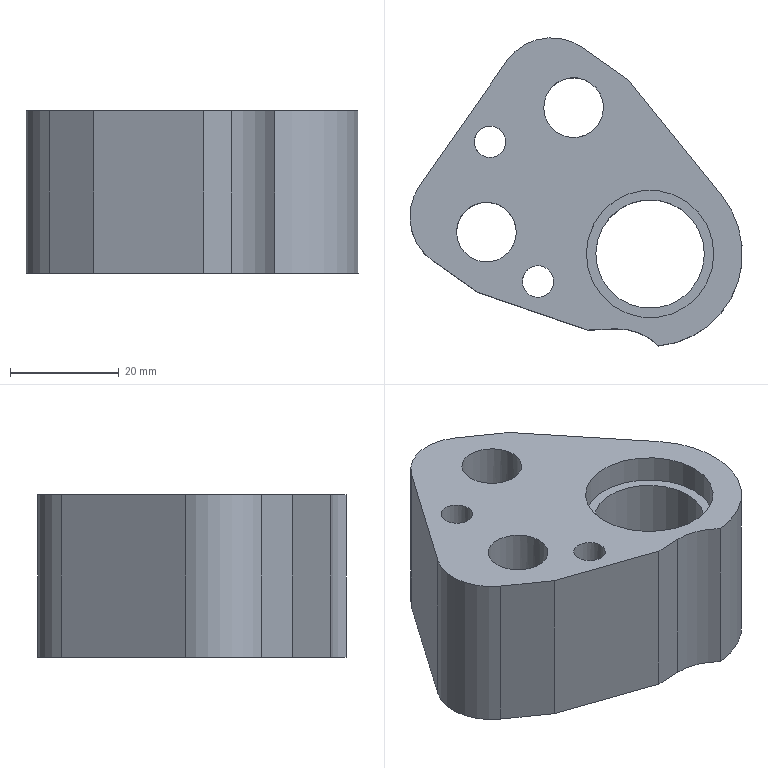Part | NX | features solid 2 | 1 solid | 27 faces | box 61.243 x 56.752 x 30 mm | volume 46658 mm3 | cylinder 14 | plane 13 | commonest cylinder face diameters 20 x3 5.8 x2 8 x2 11 x2 17 x2 21 x1
STEP:
#1=CARTESIAN_POINT('',(534.756,-127.127,74.));
#2=VERTEX_POINT('',#1);
#3=CARTESIAN_POINT('',(517.287,-105.544,74.));
#4=VERTEX_POINT('',#3);
#5=CARTESIAN_POINT('',(529.87,-121.089,74.));
#6=DIRECTION('',(-0.6291,0.7773,0.));
#7=VECTOR('',#6,1000.);
#8=LINE('',#5,#7);
#9=EDGE_CURVE('',#2,#4,#8,.T.);
#10=ORIENTED_EDGE('',*,*,#9,.F.);
#11=CARTESIAN_POINT('',(534.756,-127.127,44.));
#12=VERTEX_POINT('',#11);
#13=CARTESIAN_POINT('',(534.756,-127.127,44.));
#14=DIRECTION('',(0.,0.,1.));
#15=VECTOR('',#14,1000.);
#16=LINE('',#13,#15);
#17=EDGE_CURVE('',#12,#2,#16,.T.);
#18=ORIENTED_EDGE('',*,*,#17,.F.);
#19=CARTESIAN_POINT('',(517.287,-105.544,44.));
#20=VERTEX_POINT('',#19);
#21=CARTESIAN_POINT('',(529.87,-121.089,44.));
#22=DIRECTION('',(0.6291,-0.7773,0.));
#23=VECTOR('',#22,1000.);
#24=LINE('',#21,#23);
#25=EDGE_CURVE('',#20,#12,#24,.T.);
#26=ORIENTED_EDGE('',*,*,#25,.F.);
#27=CARTESIAN_POINT('',(517.287,-105.544,44.));
#28=DIRECTION('',(0.,0.,1.));
#29=VECTOR('',#28,1000.);
#30=LINE('',#27,#29);
#31=EDGE_CURVE('',#20,#4,#30,.T.);
#32=ORIENTED_EDGE('',*,*,#31,.T.);
#33=EDGE_LOOP('',(#10,#18,#26,#32));
#34=FACE_BOUND('',#33,.T.);
#35=CARTESIAN_POINT('',(529.87,-121.089,44.));
#36=DIRECTION('',(-0.7773,-0.6291,0.));
#37=DIRECTION('',(0.,0.,-1.));
#38=AXIS2_PLACEMENT_3D('',#35,#36,#37);
#39=PLANE('',#38);
#40=ADVANCED_FACE('',(#34),#39,.F.);
#41=CARTESIAN_POINT('',(515.152,-151.612,74.));
#42=VERTEX_POINT('',#41);
#43=CARTESIAN_POINT('',(510.031,-151.839,74.));
#44=VERTEX_POINT('',#43);
#45=CARTESIAN_POINT('',(515.285,-151.606,74.));
#46=DIRECTION('',(-0.999,-0.04437,0.));
#47=VECTOR('',#46,1000.);
#48=LINE('',#45,#47);
#49=EDGE_CURVE('',#42,#44,#48,.T.);
#50=ORIENTED_EDGE('',*,*,#49,.F.);
#51=CARTESIAN_POINT('',(523.093,-154.751,74.));
#52=VERTEX_POINT('',#51);
#53=CARTESIAN_POINT('',(515.596,-162.103,74.));
#54=DIRECTION('',(0.,0.,1.));
#55=DIRECTION('',(1.,0.,0.));
#56=AXIS2_PLACEMENT_3D('',#53,#54,#55);
#57=CIRCLE('',#56,10.5);
#58=EDGE_CURVE('',#52,#42,#57,.T.);
#59=ORIENTED_EDGE('',*,*,#58,.F.);
#60=CARTESIAN_POINT('',(521.542,-137.822,74.));
#61=DIRECTION('',(0.,0.,-1.));
#62=DIRECTION('',(0.5736,0.8192,0.));
#63=AXIS2_PLACEMENT_3D('',#60,#61,#62);
#64=CIRCLE('',#63,17.);
#65=EDGE_CURVE('',#2,#52,#64,.T.);
#66=ORIENTED_EDGE('',*,*,#65,.F.);
#67=ORIENTED_EDGE('',*,*,#9,.T.);
#68=CARTESIAN_POINT('',(509.095,-99.808,74.));
#69=VERTEX_POINT('',#68);
#70=CARTESIAN_POINT('',(528.218,-113.198,74.));
#71=DIRECTION('',(0.8192,-0.5736,0.));
#72=VECTOR('',#71,1000.);
#73=LINE('',#70,#72);
#74=EDGE_CURVE('',#69,#4,#73,.T.);
#75=ORIENTED_EDGE('',*,*,#74,.F.);
#76=CARTESIAN_POINT('',(495.168,-102.264,74.));
#77=VERTEX_POINT('',#76);
#78=CARTESIAN_POINT('',(503.359,-107.999,74.));
#79=DIRECTION('',(0.,0.,1.));
#80=DIRECTION('',(0.9397,0.342,0.));
#81=AXIS2_PLACEMENT_3D('',#78,#79,#80);
#82=CIRCLE('',#81,10.);
#83=EDGE_CURVE('',#69,#77,#82,.T.);
#84=ORIENTED_EDGE('',*,*,#83,.T.);
#85=CARTESIAN_POINT('',(479.108,-125.2,74.));
#86=VERTEX_POINT('',#85);
#87=CARTESIAN_POINT('',(487.138,-113.732,74.));
#88=DIRECTION('',(0.5736,0.8192,0.));
#89=VECTOR('',#88,1000.);
#90=LINE('',#87,#89);
#91=EDGE_CURVE('',#86,#77,#90,.T.);
#92=ORIENTED_EDGE('',*,*,#91,.F.);
#93=CARTESIAN_POINT('',(481.564,-139.127,74.));
#94=VERTEX_POINT('',#93);
#95=CARTESIAN_POINT('',(487.299,-130.936,74.));
#96=DIRECTION('',(0.,0.,1.));
#97=DIRECTION('',(0.9397,0.342,0.));
#98=AXIS2_PLACEMENT_3D('',#95,#96,#97);
#99=CIRCLE('',#98,10.);
#100=EDGE_CURVE('',#86,#94,#99,.T.);
#101=ORIENTED_EDGE('',*,*,#100,.T.);
#102=CARTESIAN_POINT('',(489.755,-144.863,74.));
#103=VERTEX_POINT('',#102);
#104=CARTESIAN_POINT('',(500.687,-152.517,74.));
#105=DIRECTION('',(-0.8192,0.5736,0.));
#106=VECTOR('',#105,1000.);
#107=LINE('',#104,#106);
#108=EDGE_CURVE('',#103,#94,#107,.T.);
#109=ORIENTED_EDGE('',*,*,#108,.F.);
#110=CARTESIAN_POINT('',(508.667,-151.37,74.));
#111=DIRECTION('',(0.9456,-0.3254,0.));
#112=VECTOR('',#111,1000.);
#113=LINE('',#110,#112);
#114=EDGE_CURVE('',#103,#44,#113,.T.);
#115=ORIENTED_EDGE('',*,*,#114,.T.);
#116=EDGE_LOOP('',(#50,#59,#66,#67,#75,#84,#92,#101,#109,#115));
#117=FACE_BOUND('',#116,.T.);
#118=CARTESIAN_POINT('',(493.716,-114.798,74.));
#119=VERTEX_POINT('',#118);
#120=CARTESIAN_POINT('',(492.053,-117.173,74.));
#121=DIRECTION('',(0.,0.,-1.));
#122=DIRECTION('',(0.5736,0.8192,0.));
#123=AXIS2_PLACEMENT_3D('',#120,#121,#122);
#124=CIRCLE('',#123,2.9);
#125=EDGE_CURVE('',#119,#119,#124,.T.);
#126=ORIENTED_EDGE('',*,*,#125,.T.);
#127=EDGE_LOOP('',(#126));
#128=FACE_BOUND('',#127,.T.);
#129=CARTESIAN_POINT('',(502.56,-140.523,74.));
#130=VERTEX_POINT('',#129);
#131=CARTESIAN_POINT('',(500.897,-142.898,74.));
#132=DIRECTION('',(0.,0.,-1.));
#133=DIRECTION('',(0.5736,0.8192,0.));
#134=AXIS2_PLACEMENT_3D('',#131,#132,#133);
#135=CIRCLE('',#134,2.9);
#136=EDGE_CURVE('',#130,#130,#135,.T.);
#137=ORIENTED_EDGE('',*,*,#136,.T.);
#138=EDGE_LOOP('',(#137));
#139=FACE_BOUND('',#138,.T.);
#140=CARTESIAN_POINT('',(494.55,-129.298,74.));
#141=VERTEX_POINT('',#140);
#142=CARTESIAN_POINT('',(491.395,-133.804,74.));
#143=DIRECTION('',(0.,0.,-1.));
#144=DIRECTION('',(0.5736,0.8192,0.));
#145=AXIS2_PLACEMENT_3D('',#142,#143,#144);
#146=CIRCLE('',#145,5.5);
#147=EDGE_CURVE('',#141,#141,#146,.T.);
#148=ORIENTED_EDGE('',*,*,#147,.T.);
#149=EDGE_LOOP('',(#148));
#150=FACE_BOUND('',#149,.T.);
#151=CARTESIAN_POINT('',(510.61,-106.362,74.));
#152=VERTEX_POINT('',#151);
#153=CARTESIAN_POINT('',(507.455,-110.867,74.));
#154=DIRECTION('',(0.,0.,-1.));
#155=DIRECTION('',(0.5736,0.8192,0.));
#156=AXIS2_PLACEMENT_3D('',#153,#154,#155);
#157=CIRCLE('',#156,5.5);
#158=EDGE_CURVE('',#152,#152,#157,.T.);
#159=ORIENTED_EDGE('',*,*,#158,.T.);
#160=EDGE_LOOP('',(#159));
#161=FACE_BOUND('',#160,.T.);
#162=CARTESIAN_POINT('',(528.282,-128.197,74.));
#163=VERTEX_POINT('',#162);
#164=CARTESIAN_POINT('',(521.542,-137.822,74.));
#165=DIRECTION('',(0.,0.,-1.));
#166=DIRECTION('',(0.5736,0.8192,0.));
#167=AXIS2_PLACEMENT_3D('',#164,#165,#166);
#168=CIRCLE('',#167,11.75);
#169=EDGE_CURVE('',#163,#163,#168,.T.);
#170=ORIENTED_EDGE('',*,*,#169,.T.);
#171=EDGE_LOOP('',(#170));
#172=FACE_BOUND('',#171,.T.);
#173=CARTESIAN_POINT('',(514.453,-132.858,74.));
#174=DIRECTION('',(0.,0.,1.));
#175=DIRECTION('',(-0.5736,-0.8192,0.));
#176=AXIS2_PLACEMENT_3D('',#173,#174,#175);
#177=PLANE('',#176);
#178=ADVANCED_FACE('',(#117,#128,#139,#150,#161,#172),#177,.T.);
#179=ORIENTED_EDGE('',*,*,#31,.F.);
#180=CARTESIAN_POINT('',(509.095,-99.808,44.));
#181=VERTEX_POINT('',#180);
#182=CARTESIAN_POINT('',(528.218,-113.198,44.));
#183=DIRECTION('',(-0.8192,0.5736,0.));
#184=VECTOR('',#183,1000.);
#185=LINE('',#182,#184);
#186=EDGE_CURVE('',#20,#181,#185,.T.);
#187=ORIENTED_EDGE('',*,*,#186,.T.);
#188=CARTESIAN_POINT('',(509.095,-99.808,44.));
#189=DIRECTION('',(0.,0.,1.));
#190=VECTOR('',#189,1000.);
#191=LINE('',#188,#190);
#192=EDGE_CURVE('',#181,#69,#191,.T.);
#193=ORIENTED_EDGE('',*,*,#192,.T.);
#194=ORIENTED_EDGE('',*,*,#74,.T.);
#195=EDGE_LOOP('',(#179,#187,#193,#194));
#196=FACE_BOUND('',#195,.T.);
#197=CARTESIAN_POINT('',(528.218,-113.198,44.));
#198=DIRECTION('',(0.5736,0.8192,0.));
#199=DIRECTION('',(0.,0.,1.));
#200=AXIS2_PLACEMENT_3D('',#197,#198,#199);
#201=PLANE('',#200);
#202=ADVANCED_FACE('',(#196),#201,.T.);
#203=CARTESIAN_POINT('',(510.031,-151.839,44.));
#204=VERTEX_POINT('',#203);
#205=CARTESIAN_POINT('',(515.152,-151.612,44.));
#206=VERTEX_POINT('',#205);
#207=CARTESIAN_POINT('',(515.285,-151.606,44.));
#208=DIRECTION('',(0.999,0.04437,0.));
#209=VECTOR('',#208,1000.);
#210=LINE('',#207,#209);
#211=EDGE_CURVE('',#204,#206,#210,.T.);
#212=ORIENTED_EDGE('',*,*,#211,.F.);
#213=CARTESIAN_POINT('',(489.755,-144.863,44.));
#214=VERTEX_POINT('',#213);
#215=CARTESIAN_POINT('',(508.667,-151.37,44.));
#216=DIRECTION('',(-0.9456,0.3254,0.));
#217=VECTOR('',#216,1000.);
#218=LINE('',#215,#217);
#219=EDGE_CURVE('',#204,#214,#218,.T.);
#220=ORIENTED_EDGE('',*,*,#219,.T.);
#221=CARTESIAN_POINT('',(481.564,-139.127,44.));
#222=VERTEX_POINT('',#221);
#223=CARTESIAN_POINT('',(500.687,-152.517,44.));
#224=DIRECTION('',(0.8192,-0.5736,0.));
#225=VECTOR('',#224,1000.);
#226=LINE('',#223,#225);
#227=EDGE_CURVE('',#222,#214,#226,.T.);
#228=ORIENTED_EDGE('',*,*,#227,.F.);
#229=CARTESIAN_POINT('',(479.108,-125.2,44.));
#230=VERTEX_POINT('',#229);
#231=CARTESIAN_POINT('',(487.299,-130.936,44.));
#232=DIRECTION('',(0.,0.,-1.));
#233=DIRECTION('',(-0.9397,-0.342,0.));
#234=AXIS2_PLACEMENT_3D('',#231,#232,#233);
#235=CIRCLE('',#234,10.);
#236=EDGE_CURVE('',#222,#230,#235,.T.);
#237=ORIENTED_EDGE('',*,*,#236,.T.);
#238=CARTESIAN_POINT('',(495.168,-102.264,44.));
#239=VERTEX_POINT('',#238);
#240=CARTESIAN_POINT('',(487.138,-113.732,44.));
#241=DIRECTION('',(-0.5736,-0.8192,0.));
#242=VECTOR('',#241,1000.);
#243=LINE('',#240,#242);
#244=EDGE_CURVE('',#239,#230,#243,.T.);
#245=ORIENTED_EDGE('',*,*,#244,.F.);
#246=CARTESIAN_POINT('',(503.359,-107.999,44.));
#247=DIRECTION('',(0.,0.,-1.));
#248=DIRECTION('',(-0.9397,-0.342,0.));
#249=AXIS2_PLACEMENT_3D('',#246,#247,#248);
#250=CIRCLE('',#249,10.);
#251=EDGE_CURVE('',#239,#181,#250,.T.);
#252=ORIENTED_EDGE('',*,*,#251,.T.);
#253=ORIENTED_EDGE('',*,*,#186,.F.);
#254=ORIENTED_EDGE('',*,*,#25,.T.);
#255=CARTESIAN_POINT('',(523.093,-154.751,44.));
#256=VERTEX_POINT('',#255);
#257=CARTESIAN_POINT('',(521.542,-137.822,44.));
#258=DIRECTION('',(0.,0.,1.));
#259=DIRECTION('',(-0.5736,-0.8192,0.));
#260=AXIS2_PLACEMENT_3D('',#257,#258,#259);
#261=CIRCLE('',#260,17.);
#262=EDGE_CURVE('',#256,#12,#261,.T.);
#263=ORIENTED_EDGE('',*,*,#262,.F.);
#264=CARTESIAN_POINT('',(515.596,-162.103,44.));
#265=DIRECTION('',(0.,0.,-1.));
#266=DIRECTION('',(-1.,0.,0.));
#267=AXIS2_PLACEMENT_3D('',#264,#265,#266);
#268=CIRCLE('',#267,10.5);
#269=EDGE_CURVE('',#206,#256,#268,.T.);
#270=ORIENTED_EDGE('',*,*,#269,.F.);
#271=EDGE_LOOP('',(#212,#220,#228,#237,#245,#252,#253,#254,#263,#270));
#272=FACE_BOUND('',#271,.T.);
#273=CARTESIAN_POINT('',(489.759,-120.45,44.));
#274=VERTEX_POINT('',#273);
#275=CARTESIAN_POINT('',(492.053,-117.173,44.));
#276=DIRECTION('',(0.,0.,1.));
#277=DIRECTION('',(-0.5736,-0.8192,0.));
#278=AXIS2_PLACEMENT_3D('',#275,#276,#277);
#279=CIRCLE('',#278,4.);
#280=EDGE_CURVE('',#274,#274,#279,.T.);
#281=ORIENTED_EDGE('',*,*,#280,.T.);
#282=EDGE_LOOP('',(#281));
#283=FACE_BOUND('',#282,.T.);
#284=CARTESIAN_POINT('',(498.603,-146.175,44.));
#285=VERTEX_POINT('',#284);
#286=CARTESIAN_POINT('',(500.897,-142.898,44.));
#287=DIRECTION('',(0.,0.,1.));
#288=DIRECTION('',(-0.5736,-0.8192,0.));
#289=AXIS2_PLACEMENT_3D('',#286,#287,#288);
#290=CIRCLE('',#289,4.);
#291=EDGE_CURVE('',#285,#285,#290,.T.);
#292=ORIENTED_EDGE('',*,*,#291,.T.);
#293=EDGE_LOOP('',(#292));
#294=FACE_BOUND('',#293,.T.);
#295=CARTESIAN_POINT('',(486.52,-140.766,44.));
#296=VERTEX_POINT('',#295);
#297=CARTESIAN_POINT('',(491.395,-133.804,44.));
#298=DIRECTION('',(0.,0.,1.));
#299=DIRECTION('',(-0.5736,-0.8192,0.));
#300=AXIS2_PLACEMENT_3D('',#297,#298,#299);
#301=CIRCLE('',#300,8.5);
#302=EDGE_CURVE('',#296,#296,#301,.T.);
#303=ORIENTED_EDGE('',*,*,#302,.T.);
#304=EDGE_LOOP('',(#303));
#305=FACE_BOUND('',#304,.T.);
#306=CARTESIAN_POINT('',(502.58,-117.83,44.));
#307=VERTEX_POINT('',#306);
#308=CARTESIAN_POINT('',(507.455,-110.867,44.));
#309=DIRECTION('',(0.,0.,1.));
#310=DIRECTION('',(-0.5736,-0.8192,0.));
#311=AXIS2_PLACEMENT_3D('',#308,#309,#310);
#312=CIRCLE('',#311,8.5);
#313=EDGE_CURVE('',#307,#307,#312,.T.);
#314=ORIENTED_EDGE('',*,*,#313,.T.);
#315=EDGE_LOOP('',(#314));
#316=FACE_BOUND('',#315,.T.);
#317=CARTESIAN_POINT('',(515.807,-146.014,44.));
#318=VERTEX_POINT('',#317);
#319=CARTESIAN_POINT('',(521.542,-137.822,44.));
#320=DIRECTION('',(0.,0.,1.));
#321=DIRECTION('',(-0.5736,-0.8192,0.));
#322=AXIS2_PLACEMENT_3D('',#319,#320,#321);
#323=CIRCLE('',#322,10.);
#324=EDGE_CURVE('',#318,#318,#323,.T.);
#325=ORIENTED_EDGE('',*,*,#324,.T.);
#326=EDGE_LOOP('',(#325));
#327=FACE_BOUND('',#326,.T.);
#328=CARTESIAN_POINT('',(514.453,-132.858,44.));
#329=DIRECTION('',(0.,0.,-1.));
#330=DIRECTION('',(0.5736,0.8192,0.));
#331=AXIS2_PLACEMENT_3D('',#328,#329,#330);
#332=PLANE('',#331);
#333=ADVANCED_FACE('',(#272,#283,#294,#305,#316,#327),#332,.T.);
#334=CARTESIAN_POINT('',(489.755,-144.863,44.));
#335=DIRECTION('',(0.,0.,1.));
#336=VECTOR('',#335,1000.);
#337=LINE('',#334,#336);
#338=EDGE_CURVE('',#214,#103,#337,.T.);
#339=ORIENTED_EDGE('',*,*,#338,.T.);
#340=ORIENTED_EDGE('',*,*,#108,.T.);
#341=CARTESIAN_POINT('',(481.564,-139.127,44.));
#342=DIRECTION('',(0.,0.,1.));
#343=VECTOR('',#342,1000.);
#344=LINE('',#341,#343);
#345=EDGE_CURVE('',#94,#222,#344,.F.);
#346=ORIENTED_EDGE('',*,*,#345,.T.);
#347=ORIENTED_EDGE('',*,*,#227,.T.);
#348=EDGE_LOOP('',(#339,#340,#346,#347));
#349=FACE_BOUND('',#348,.T.);
#350=CARTESIAN_POINT('',(500.687,-152.517,44.));
#351=DIRECTION('',(-0.5736,-0.8192,0.));
#352=DIRECTION('',(0.,0.,-1.));
#353=AXIS2_PLACEMENT_3D('',#350,#351,#352);
#354=PLANE('',#353);
#355=ADVANCED_FACE('',(#349),#354,.T.);
#356=CARTESIAN_POINT('',(523.093,-154.751,250.));
#357=DIRECTION('',(0.,0.,1.));
#358=VECTOR('',#357,1000.);
#359=LINE('',#356,#358);
#360=EDGE_CURVE('',#256,#52,#359,.T.);
#361=ORIENTED_EDGE('',*,*,#360,.F.);
#362=ORIENTED_EDGE('',*,*,#262,.T.);
#363=ORIENTED_EDGE('',*,*,#17,.T.);
#364=ORIENTED_EDGE('',*,*,#65,.T.);
#365=EDGE_LOOP('',(#361,#362,#363,#364));
#366=FACE_BOUND('',#365,.T.);
#367=CARTESIAN_POINT('',(521.542,-137.822,74.));
#368=DIRECTION('',(0.,0.,-1.));
#369=DIRECTION('',(0.5736,0.8192,0.));
#370=AXIS2_PLACEMENT_3D('',#367,#368,#369);
#371=CYLINDRICAL_SURFACE('',#370,17.);
#372=ADVANCED_FACE('',(#366),#371,.T.);
#373=ORIENTED_EDGE('',*,*,#244,.T.);
#374=CARTESIAN_POINT('',(479.108,-125.2,44.));
#375=DIRECTION('',(0.,0.,1.));
#376=VECTOR('',#375,1000.);
#377=LINE('',#374,#376);
#378=EDGE_CURVE('',#230,#86,#377,.T.);
#379=ORIENTED_EDGE('',*,*,#378,.T.);
#380=ORIENTED_EDGE('',*,*,#91,.T.);
#381=CARTESIAN_POINT('',(495.168,-102.264,44.));
#382=DIRECTION('',(0.,0.,1.));
#383=VECTOR('',#382,1000.);
#384=LINE('',#381,#383);
#385=EDGE_CURVE('',#77,#239,#384,.F.);
#386=ORIENTED_EDGE('',*,*,#385,.T.);
#387=EDGE_LOOP('',(#373,#379,#380,#386));
#388=FACE_BOUND('',#387,.T.);
#389=CARTESIAN_POINT('',(487.138,-113.732,44.));
#390=DIRECTION('',(-0.8192,0.5736,0.));
#391=DIRECTION('',(0.,0.,-1.));
#392=AXIS2_PLACEMENT_3D('',#389,#390,#391);
#393=PLANE('',#392);
#394=ADVANCED_FACE('',(#388),#393,.T.);
#395=CARTESIAN_POINT('',(527.278,-129.631,69.));
#396=VERTEX_POINT('',#395);
#397=CARTESIAN_POINT('',(521.542,-137.822,69.));
#398=DIRECTION('',(0.,0.,-1.));
#399=DIRECTION('',(0.5736,0.8192,0.));
#400=AXIS2_PLACEMENT_3D('',#397,#398,#399);
#401=CIRCLE('',#400,10.);
#402=EDGE_CURVE('',#396,#396,#401,.T.);
#403=ORIENTED_EDGE('',*,*,#402,.T.);
#404=EDGE_LOOP('',(#403));
#405=FACE_BOUND('',#404,.T.);
#406=CARTESIAN_POINT('',(514.803,-147.447,69.));
#407=VERTEX_POINT('',#406);
#408=CARTESIAN_POINT('',(521.542,-137.822,69.));
#409=DIRECTION('',(0.,0.,1.));
#410=DIRECTION('',(-0.5736,-0.8192,0.));
#411=AXIS2_PLACEMENT_3D('',#408,#409,#410);
#412=CIRCLE('',#411,11.75);
#413=EDGE_CURVE('',#407,#407,#412,.T.);
#414=ORIENTED_EDGE('',*,*,#413,.T.);
#415=EDGE_LOOP('',(#414));
#416=FACE_BOUND('',#415,.T.);
#417=CARTESIAN_POINT('',(521.542,-137.822,69.));
#418=DIRECTION('',(0.,0.,-1.));
#419=DIRECTION('',(0.5736,0.8192,0.));
#420=AXIS2_PLACEMENT_3D('',#417,#418,#419);
#421=PLANE('',#420);
#422=ADVANCED_FACE('',(#405,#416),#421,.F.);
#423=ORIENTED_EDGE('',*,*,#413,.F.);
#424=EDGE_LOOP('',(#423));
#425=FACE_BOUND('',#424,.T.);
#426=ORIENTED_EDGE('',*,*,#169,.F.);
#427=EDGE_LOOP('',(#426));
#428=FACE_BOUND('',#427,.T.);
#429=CARTESIAN_POINT('',(521.542,-137.822,74.));
#430=DIRECTION('',(0.,0.,-1.));
#431=DIRECTION('',(0.5736,0.8192,0.));
#432=AXIS2_PLACEMENT_3D('',#429,#430,#431);
#433=CYLINDRICAL_SURFACE('',#432,11.75);
#434=ADVANCED_FACE('',(#425,#428),#433,.F.);
#435=ORIENTED_EDGE('',*,*,#324,.F.);
#436=EDGE_LOOP('',(#435));
#437=FACE_BOUND('',#436,.T.);
#438=ORIENTED_EDGE('',*,*,#402,.F.);
#439=EDGE_LOOP('',(#438));
#440=FACE_BOUND('',#439,.T.);
#441=CARTESIAN_POINT('',(521.542,-137.822,69.));
#442=DIRECTION('',(0.,0.,-1.));
#443=DIRECTION('',(0.5736,0.8192,0.));
#444=AXIS2_PLACEMENT_3D('',#441,#442,#443);
#445=CYLINDRICAL_SURFACE('',#444,10.);
#446=ADVANCED_FACE('',(#437,#440),#445,.F.);
#447=CARTESIAN_POINT('',(512.624,-108.986,56.));
#448=VERTEX_POINT('',#447);
#449=CARTESIAN_POINT('',(507.455,-110.867,56.));
#450=DIRECTION('',(0.,0.,1.));
#451=DIRECTION('',(0.9397,0.342,0.));
#452=AXIS2_PLACEMENT_3D('',#449,#450,#451);
#453=CIRCLE('',#452,5.5);
#454=EDGE_CURVE('',#448,#448,#453,.F.);
#455=ORIENTED_EDGE('',*,*,#454,.T.);
#456=EDGE_LOOP('',(#455));
#457=FACE_BOUND('',#456,.T.);
#458=ORIENTED_EDGE('',*,*,#158,.F.);
#459=EDGE_LOOP('',(#458));
#460=FACE_BOUND('',#459,.T.);
#461=CARTESIAN_POINT('',(507.455,-110.867,74.));
#462=DIRECTION('',(0.,0.,-1.));
#463=DIRECTION('',(0.5736,0.8192,0.));
#464=AXIS2_PLACEMENT_3D('',#461,#462,#463);
#465=CYLINDRICAL_SURFACE('',#464,5.5);
#466=ADVANCED_FACE('',(#457,#460),#465,.F.);
#467=CARTESIAN_POINT('',(512.331,-103.905,56.));
#468=VERTEX_POINT('',#467);
#469=CARTESIAN_POINT('',(507.455,-110.867,56.));
#470=DIRECTION('',(0.,0.,-1.));
#471=DIRECTION('',(0.5736,0.8192,0.));
#472=AXIS2_PLACEMENT_3D('',#469,#470,#471);
#473=CIRCLE('',#472,8.5);
#474=EDGE_CURVE('',#468,#468,#473,.T.);
#475=ORIENTED_EDGE('',*,*,#474,.T.);
#476=EDGE_LOOP('',(#475));
#477=FACE_BOUND('',#476,.T.);
#478=ORIENTED_EDGE('',*,*,#454,.F.);
#479=EDGE_LOOP('',(#478));
#480=FACE_BOUND('',#479,.T.);
#481=CARTESIAN_POINT('',(507.455,-110.867,56.));
#482=DIRECTION('',(0.,0.,1.));
#483=DIRECTION('',(-0.5736,-0.8192,0.));
#484=AXIS2_PLACEMENT_3D('',#481,#482,#483);
#485=PLANE('',#484);
#486=ADVANCED_FACE('',(#477,#480),#485,.F.);
#487=ORIENTED_EDGE('',*,*,#313,.F.);
#488=EDGE_LOOP('',(#487));
#489=FACE_BOUND('',#488,.T.);
#490=ORIENTED_EDGE('',*,*,#474,.F.);
#491=EDGE_LOOP('',(#490));
#492=FACE_BOUND('',#491,.T.);
#493=CARTESIAN_POINT('',(507.455,-110.867,56.));
#494=DIRECTION('',(0.,0.,-1.));
#495=DIRECTION('',(0.5736,0.8192,0.));
#496=AXIS2_PLACEMENT_3D('',#493,#494,#495);
#497=CYLINDRICAL_SURFACE('',#496,8.5);
#498=ADVANCED_FACE('',(#489,#492),#497,.F.);
#499=CARTESIAN_POINT('',(496.563,-131.923,56.));
#500=VERTEX_POINT('',#499);
#501=CARTESIAN_POINT('',(491.395,-133.804,56.));
#502=DIRECTION('',(0.,0.,1.));
#503=DIRECTION('',(0.9397,0.342,0.));
#504=AXIS2_PLACEMENT_3D('',#501,#502,#503);
#505=CIRCLE('',#504,5.5);
#506=EDGE_CURVE('',#500,#500,#505,.F.);
#507=ORIENTED_EDGE('',*,*,#506,.T.);
#508=EDGE_LOOP('',(#507));
#509=FACE_BOUND('',#508,.T.);
#510=ORIENTED_EDGE('',*,*,#147,.F.);
#511=EDGE_LOOP('',(#510));
#512=FACE_BOUND('',#511,.T.);
#513=CARTESIAN_POINT('',(491.395,-133.804,74.));
#514=DIRECTION('',(0.,0.,-1.));
#515=DIRECTION('',(0.5736,0.8192,0.));
#516=AXIS2_PLACEMENT_3D('',#513,#514,#515);
#517=CYLINDRICAL_SURFACE('',#516,5.5);
#518=ADVANCED_FACE('',(#509,#512),#517,.F.);
#519=CARTESIAN_POINT('',(496.271,-126.841,56.));
#520=VERTEX_POINT('',#519);
#521=CARTESIAN_POINT('',(491.395,-133.804,56.));
#522=DIRECTION('',(0.,0.,-1.));
#523=DIRECTION('',(0.5736,0.8192,0.));
#524=AXIS2_PLACEMENT_3D('',#521,#522,#523);
#525=CIRCLE('',#524,8.5);
#526=EDGE_CURVE('',#520,#520,#525,.T.);
#527=ORIENTED_EDGE('',*,*,#526,.T.);
#528=EDGE_LOOP('',(#527));
#529=FACE_BOUND('',#528,.T.);
#530=ORIENTED_EDGE('',*,*,#506,.F.);
#531=EDGE_LOOP('',(#530));
#532=FACE_BOUND('',#531,.T.);
#533=CARTESIAN_POINT('',(491.395,-133.804,56.));
#534=DIRECTION('',(0.,0.,1.));
#535=DIRECTION('',(-0.5736,-0.8192,0.));
#536=AXIS2_PLACEMENT_3D('',#533,#534,#535);
#537=PLANE('',#536);
#538=ADVANCED_FACE('',(#529,#532),#537,.F.);
#539=ORIENTED_EDGE('',*,*,#302,.F.);
#540=EDGE_LOOP('',(#539));
#541=FACE_BOUND('',#540,.T.);
#542=ORIENTED_EDGE('',*,*,#526,.F.);
#543=EDGE_LOOP('',(#542));
#544=FACE_BOUND('',#543,.T.);
#545=CARTESIAN_POINT('',(491.395,-133.804,56.));
#546=DIRECTION('',(0.,0.,-1.));
#547=DIRECTION('',(0.5736,0.8192,0.));
#548=AXIS2_PLACEMENT_3D('',#545,#546,#547);
#549=CYLINDRICAL_SURFACE('',#548,8.5);
#550=ADVANCED_FACE('',(#541,#544),#549,.F.);
#551=CARTESIAN_POINT('',(503.622,-141.907,64.));
#552=VERTEX_POINT('',#551);
#553=CARTESIAN_POINT('',(500.897,-142.898,64.));
#554=DIRECTION('',(0.,0.,1.));
#555=DIRECTION('',(0.9397,0.342,0.));
#556=AXIS2_PLACEMENT_3D('',#553,#554,#555);
#557=CIRCLE('',#556,2.9);
#558=EDGE_CURVE('',#552,#552,#557,.F.);
#559=ORIENTED_EDGE('',*,*,#558,.T.);
#560=EDGE_LOOP('',(#559));
#561=FACE_BOUND('',#560,.T.);
#562=ORIENTED_EDGE('',*,*,#136,.F.);
#563=EDGE_LOOP('',(#562));
#564=FACE_BOUND('',#563,.T.);
#565=CARTESIAN_POINT('',(500.897,-142.898,74.));
#566=DIRECTION('',(0.,0.,-1.));
#567=DIRECTION('',(0.5736,0.8192,0.));
#568=AXIS2_PLACEMENT_3D('',#565,#566,#567);
#569=CYLINDRICAL_SURFACE('',#568,2.9);
#570=ADVANCED_FACE('',(#561,#564),#569,.F.);
#571=CARTESIAN_POINT('',(503.191,-139.622,64.));
#572=VERTEX_POINT('',#571);
#573=CARTESIAN_POINT('',(500.897,-142.898,64.));
#574=DIRECTION('',(0.,0.,-1.));
#575=DIRECTION('',(0.5736,0.8192,0.));
#576=AXIS2_PLACEMENT_3D('',#573,#574,#575);
#577=CIRCLE('',#576,4.);
#578=EDGE_CURVE('',#572,#572,#577,.T.);
#579=ORIENTED_EDGE('',*,*,#578,.T.);
#580=EDGE_LOOP('',(#579));
#581=FACE_BOUND('',#580,.T.);
#582=ORIENTED_EDGE('',*,*,#558,.F.);
#583=EDGE_LOOP('',(#582));
#584=FACE_BOUND('',#583,.T.);
#585=CARTESIAN_POINT('',(500.897,-142.898,64.));
#586=DIRECTION('',(0.,0.,1.));
#587=DIRECTION('',(-0.5736,-0.8192,0.));
#588=AXIS2_PLACEMENT_3D('',#585,#586,#587);
#589=PLANE('',#588);
#590=ADVANCED_FACE('',(#581,#584),#589,.F.);
#591=ORIENTED_EDGE('',*,*,#291,.F.);
#592=EDGE_LOOP('',(#591));
#593=FACE_BOUND('',#592,.T.);
#594=ORIENTED_EDGE('',*,*,#578,.F.);
#595=EDGE_LOOP('',(#594));
#596=FACE_BOUND('',#595,.T.);
#597=CARTESIAN_POINT('',(500.897,-142.898,64.));
#598=DIRECTION('',(0.,0.,-1.));
#599=DIRECTION('',(0.5736,0.8192,0.));
#600=AXIS2_PLACEMENT_3D('',#597,#598,#599);
#601=CYLINDRICAL_SURFACE('',#600,4.);
#602=ADVANCED_FACE('',(#593,#596),#601,.F.);
#603=CARTESIAN_POINT('',(494.778,-116.181,64.));
#604=VERTEX_POINT('',#603);
#605=CARTESIAN_POINT('',(492.053,-117.173,64.));
#606=DIRECTION('',(0.,0.,1.));
#607=DIRECTION('',(0.9397,0.342,0.));
#608=AXIS2_PLACEMENT_3D('',#605,#606,#607);
#609=CIRCLE('',#608,2.9);
#610=EDGE_CURVE('',#604,#604,#609,.F.);
#611=ORIENTED_EDGE('',*,*,#610,.T.);
#612=EDGE_LOOP('',(#611));
#613=FACE_BOUND('',#612,.T.);
#614=ORIENTED_EDGE('',*,*,#125,.F.);
#615=EDGE_LOOP('',(#614));
#616=FACE_BOUND('',#615,.T.);
#617=CARTESIAN_POINT('',(492.053,-117.173,74.));
#618=DIRECTION('',(0.,0.,-1.));
#619=DIRECTION('',(0.5736,0.8192,0.));
#620=AXIS2_PLACEMENT_3D('',#617,#618,#619);
#621=CYLINDRICAL_SURFACE('',#620,2.9);
#622=ADVANCED_FACE('',(#613,#616),#621,.F.);
#623=CARTESIAN_POINT('',(494.347,-113.897,64.));
#624=VERTEX_POINT('',#623);
#625=CARTESIAN_POINT('',(492.053,-117.173,64.));
#626=DIRECTION('',(0.,0.,-1.));
#627=DIRECTION('',(0.5736,0.8192,0.));
#628=AXIS2_PLACEMENT_3D('',#625,#626,#627);
#629=CIRCLE('',#628,4.);
#630=EDGE_CURVE('',#624,#624,#629,.T.);
#631=ORIENTED_EDGE('',*,*,#630,.T.);
#632=EDGE_LOOP('',(#631));
#633=FACE_BOUND('',#632,.T.);
#634=ORIENTED_EDGE('',*,*,#610,.F.);
#635=EDGE_LOOP('',(#634));
#636=FACE_BOUND('',#635,.T.);
#637=CARTESIAN_POINT('',(492.053,-117.173,64.));
#638=DIRECTION('',(0.,0.,1.));
#639=DIRECTION('',(-0.5736,-0.8192,0.));
#640=AXIS2_PLACEMENT_3D('',#637,#638,#639);
#641=PLANE('',#640);
#642=ADVANCED_FACE('',(#633,#636),#641,.F.);
#643=ORIENTED_EDGE('',*,*,#280,.F.);
#644=EDGE_LOOP('',(#643));
#645=FACE_BOUND('',#644,.T.);
#646=ORIENTED_EDGE('',*,*,#630,.F.);
#647=EDGE_LOOP('',(#646));
#648=FACE_BOUND('',#647,.T.);
#649=CARTESIAN_POINT('',(492.053,-117.173,64.));
#650=DIRECTION('',(0.,0.,-1.));
#651=DIRECTION('',(0.5736,0.8192,0.));
#652=AXIS2_PLACEMENT_3D('',#649,#650,#651);
#653=CYLINDRICAL_SURFACE('',#652,4.);
#654=ADVANCED_FACE('',(#645,#648),#653,.F.);
#655=ORIENTED_EDGE('',*,*,#236,.F.);
#656=ORIENTED_EDGE('',*,*,#345,.F.);
#657=ORIENTED_EDGE('',*,*,#100,.F.);
#658=ORIENTED_EDGE('',*,*,#378,.F.);
#659=EDGE_LOOP('',(#655,#656,#657,#658));
#660=FACE_BOUND('',#659,.T.);
#661=CARTESIAN_POINT('',(487.299,-130.936,44.));
#662=DIRECTION('',(0.,0.,1.));
#663=DIRECTION('',(0.9397,0.342,0.));
#664=AXIS2_PLACEMENT_3D('',#661,#662,#663);
#665=CYLINDRICAL_SURFACE('',#664,10.);
#666=ADVANCED_FACE('',(#660),#665,.T.);
#667=ORIENTED_EDGE('',*,*,#251,.F.);
#668=ORIENTED_EDGE('',*,*,#385,.F.);
#669=ORIENTED_EDGE('',*,*,#83,.F.);
#670=ORIENTED_EDGE('',*,*,#192,.F.);
#671=EDGE_LOOP('',(#667,#668,#669,#670));
#672=FACE_BOUND('',#671,.T.);
#673=CARTESIAN_POINT('',(503.359,-107.999,44.));
#674=DIRECTION('',(0.,0.,1.));
#675=DIRECTION('',(0.9397,0.342,0.));
#676=AXIS2_PLACEMENT_3D('',#673,#674,#675);
#677=CYLINDRICAL_SURFACE('',#676,10.);
#678=ADVANCED_FACE('',(#672),#677,.T.);
#679=ORIENTED_EDGE('',*,*,#219,.F.);
#680=CARTESIAN_POINT('',(510.031,-151.839,44.));
#681=DIRECTION('',(0.,0.,1.));
#682=VECTOR('',#681,1000.);
#683=LINE('',#680,#682);
#684=EDGE_CURVE('',#204,#44,#683,.T.);
#685=ORIENTED_EDGE('',*,*,#684,.T.);
#686=ORIENTED_EDGE('',*,*,#114,.F.);
#687=ORIENTED_EDGE('',*,*,#338,.F.);
#688=EDGE_LOOP('',(#679,#685,#686,#687));
#689=FACE_BOUND('',#688,.T.);
#690=CARTESIAN_POINT('',(508.667,-151.37,44.));
#691=DIRECTION('',(0.3254,0.9456,0.));
#692=DIRECTION('',(0.,0.,1.));
#693=AXIS2_PLACEMENT_3D('',#690,#691,#692);
#694=PLANE('',#693);
#695=ADVANCED_FACE('',(#689),#694,.F.);
#696=ORIENTED_EDGE('',*,*,#360,.T.);
#697=ORIENTED_EDGE('',*,*,#58,.T.);
#698=CARTESIAN_POINT('',(515.152,-151.612,0.));
#699=DIRECTION('',(0.,0.,1.));
#700=VECTOR('',#699,1000.);
#701=LINE('',#698,#700);
#702=EDGE_CURVE('',#206,#42,#701,.T.);
#703=ORIENTED_EDGE('',*,*,#702,.F.);
#704=ORIENTED_EDGE('',*,*,#269,.T.);
#705=EDGE_LOOP('',(#696,#697,#703,#704));
#706=FACE_BOUND('',#705,.T.);
#707=CARTESIAN_POINT('',(515.596,-162.103,0.));
#708=DIRECTION('',(0.,0.,1.));
#709=DIRECTION('',(1.,0.,0.));
#710=AXIS2_PLACEMENT_3D('',#707,#708,#709);
#711=CYLINDRICAL_SURFACE('',#710,10.5);
#712=ADVANCED_FACE('',(#706),#711,.F.);
#713=ORIENTED_EDGE('',*,*,#702,.T.);
#714=ORIENTED_EDGE('',*,*,#49,.T.);
#715=ORIENTED_EDGE('',*,*,#684,.F.);
#716=ORIENTED_EDGE('',*,*,#211,.T.);
#717=EDGE_LOOP('',(#713,#714,#715,#716));
#718=FACE_BOUND('',#717,.T.);
#719=CARTESIAN_POINT('',(515.152,-151.612,0.));
#720=DIRECTION('',(-0.04437,0.999,0.));
#721=DIRECTION('',(-0.999,-0.04437,0.));
#722=AXIS2_PLACEMENT_3D('',#719,#720,#721);
#723=PLANE('',#722);
#724=ADVANCED_FACE('',(#718),#723,.F.);
#725=CLOSED_SHELL('',(#40,#178,#202,#333,#355,#372,#394,#422,#434,#446,#466,#486,#498,#518,#538,#550,#570,#590,#602,#622,#642,#654,#666,#678,#695,#712,#724));
#726=MANIFOLD_SOLID_BREP('',#725);
#727=(LENGTH_UNIT()NAMED_UNIT(*)SI_UNIT(.MILLI.,.METRE.));
#728=UNCERTAINTY_MEASURE_WITH_UNIT(LENGTH_MEASURE(0.00001),#727,'','');
#729=(NAMED_UNIT(*)PLANE_ANGLE_UNIT()SI_UNIT($,.RADIAN.));
#730=(NAMED_UNIT(*)SI_UNIT($,.STERADIAN.)SOLID_ANGLE_UNIT());
#731=(GEOMETRIC_REPRESENTATION_CONTEXT(3)GLOBAL_UNCERTAINTY_ASSIGNED_CONTEXT((#728))GLOBAL_UNIT_ASSIGNED_CONTEXT((#727,#729,#730))REPRESENTATION_CONTEXT('',''));
#732=ADVANCED_BREP_SHAPE_REPRESENTATION('',(#726),#731);